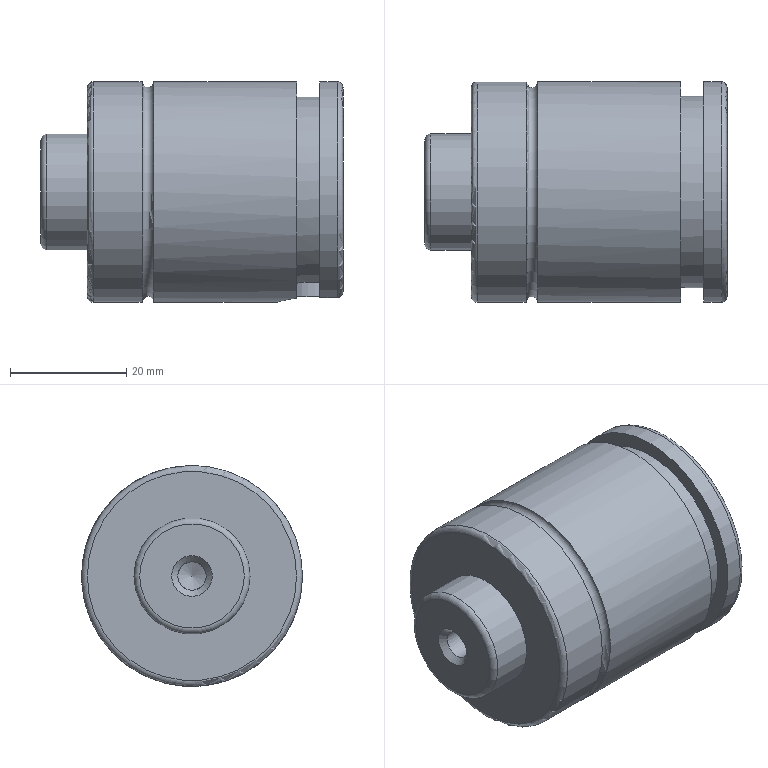Part | NX | features 1 2 | 1 solid | 34 faces | box 52 x 38 x 38 mm | volume 50464 mm3 | plane 16 | cylinder 10 | torus 4 | cone 4 | commonest cylinder face diameters 4.9 x3 38 x3 9.5 x1 11 x1 20 x1 33 x1
STEP:
#1=CARTESIAN_POINT('',(-1488.5,-459.,-300.));
#2=VERTEX_POINT('',#1);
#3=CARTESIAN_POINT('',(-1488.5,-440.,-300.));
#4=DIRECTION('',(1.,0.,0.));
#5=DIRECTION('',(0.,-1.,0.));
#6=AXIS2_PLACEMENT_3D('',#3,#4,#5);
#7=CIRCLE('',#6,19.);
#8=EDGE_CURVE('',#2,#2,#7,.T.);
#9=ORIENTED_EDGE('',*,*,#8,.F.);
#10=EDGE_LOOP('',(#9));
#11=FACE_BOUND('',#10,.T.);
#12=CARTESIAN_POINT('',(-1490.5,-459.,-300.));
#13=VERTEX_POINT('',#12);
#14=CARTESIAN_POINT('',(-1490.5,-440.,-300.));
#15=DIRECTION('',(1.,0.,0.));
#16=DIRECTION('',(0.,-1.,0.));
#17=AXIS2_PLACEMENT_3D('',#14,#15,#16);
#18=CIRCLE('',#17,19.);
#19=EDGE_CURVE('',#13,#13,#18,.T.);
#20=ORIENTED_EDGE('',*,*,#19,.T.);
#21=EDGE_LOOP('',(#20));
#22=FACE_BOUND('',#21,.T.);
#23=CARTESIAN_POINT('',(-1489.5,-440.,-300.));
#24=DIRECTION('',(-1.,0.,0.));
#25=DIRECTION('',(0.,0.,1.));
#26=AXIS2_PLACEMENT_3D('',#23,#24,#25);
#27=TOROIDAL_SURFACE('',#26,19.,1.);
#28=ADVANCED_FACE('',(#11,#22),#27,.F.);
#29=CARTESIAN_POINT('',(-1498.9,-459.,-300.));
#30=VERTEX_POINT('',#29);
#31=CARTESIAN_POINT('',(-1498.9,-440.,-300.));
#32=DIRECTION('',(1.,0.,0.));
#33=DIRECTION('',(0.,-1.,0.));
#34=AXIS2_PLACEMENT_3D('',#31,#32,#33);
#35=CIRCLE('',#34,19.);
#36=EDGE_CURVE('',#30,#30,#35,.T.);
#37=ORIENTED_EDGE('',*,*,#36,.F.);
#38=EDGE_LOOP('',(#37));
#39=FACE_BOUND('',#38,.T.);
#40=CARTESIAN_POINT('',(-1499.9,-458.,-300.));
#41=VERTEX_POINT('',#40);
#42=CARTESIAN_POINT('',(-1499.9,-440.,-300.));
#43=DIRECTION('',(1.,0.,0.));
#44=DIRECTION('',(0.,-1.,0.));
#45=AXIS2_PLACEMENT_3D('',#42,#43,#44);
#46=CIRCLE('',#45,18.);
#47=EDGE_CURVE('',#41,#41,#46,.T.);
#48=ORIENTED_EDGE('',*,*,#47,.T.);
#49=EDGE_LOOP('',(#48));
#50=FACE_BOUND('',#49,.T.);
#51=CARTESIAN_POINT('',(-1498.9,-440.,-300.));
#52=DIRECTION('',(-1.,0.,0.));
#53=DIRECTION('',(0.,0.,1.));
#54=AXIS2_PLACEMENT_3D('',#51,#52,#53);
#55=TOROIDAL_SURFACE('',#54,18.,1.);
#56=ADVANCED_FACE('',(#39,#50),#55,.T.);
#57=ORIENTED_EDGE('',*,*,#19,.F.);
#58=EDGE_LOOP('',(#57));
#59=FACE_BOUND('',#58,.T.);
#60=ORIENTED_EDGE('',*,*,#36,.T.);
#61=EDGE_LOOP('',(#60));
#62=FACE_BOUND('',#61,.T.);
#63=CARTESIAN_POINT('',(-1494.7,-440.,-300.));
#64=DIRECTION('',(1.,0.,0.));
#65=DIRECTION('',(0.,0.,-1.));
#66=AXIS2_PLACEMENT_3D('',#63,#64,#65);
#67=CYLINDRICAL_SURFACE('',#66,19.);
#68=ADVANCED_FACE('',(#59,#62),#67,.T.);
#69=CARTESIAN_POINT('',(-1506.9,-450.,-300.));
#70=VERTEX_POINT('',#69);
#71=CARTESIAN_POINT('',(-1506.9,-440.,-300.));
#72=DIRECTION('',(1.,0.,0.));
#73=DIRECTION('',(0.,-1.,0.));
#74=AXIS2_PLACEMENT_3D('',#71,#72,#73);
#75=CIRCLE('',#74,10.);
#76=EDGE_CURVE('',#70,#70,#75,.T.);
#77=ORIENTED_EDGE('',*,*,#76,.F.);
#78=EDGE_LOOP('',(#77));
#79=FACE_BOUND('',#78,.T.);
#80=CARTESIAN_POINT('',(-1507.9,-449.,-300.));
#81=VERTEX_POINT('',#80);
#82=CARTESIAN_POINT('',(-1507.9,-440.,-300.));
#83=DIRECTION('',(1.,0.,0.));
#84=DIRECTION('',(0.,-1.,0.));
#85=AXIS2_PLACEMENT_3D('',#82,#83,#84);
#86=CIRCLE('',#85,9.);
#87=EDGE_CURVE('',#81,#81,#86,.T.);
#88=ORIENTED_EDGE('',*,*,#87,.T.);
#89=EDGE_LOOP('',(#88));
#90=FACE_BOUND('',#89,.T.);
#91=CARTESIAN_POINT('',(-1506.9,-440.,-300.));
#92=DIRECTION('',(-1.,0.,0.));
#93=DIRECTION('',(0.,0.,1.));
#94=AXIS2_PLACEMENT_3D('',#91,#92,#93);
#95=TOROIDAL_SURFACE('',#94,9.,1.);
#96=ADVANCED_FACE('',(#79,#90),#95,.T.);
#97=CARTESIAN_POINT('',(-1499.9,-450.,-300.));
#98=VERTEX_POINT('',#97);
#99=CARTESIAN_POINT('',(-1499.9,-440.,-300.));
#100=DIRECTION('',(-1.,0.,0.));
#101=DIRECTION('',(0.,-1.,0.));
#102=AXIS2_PLACEMENT_3D('',#99,#100,#101);
#103=CIRCLE('',#102,10.);
#104=EDGE_CURVE('',#98,#98,#103,.T.);
#105=ORIENTED_EDGE('',*,*,#104,.T.);
#106=EDGE_LOOP('',(#105));
#107=FACE_BOUND('',#106,.T.);
#108=ORIENTED_EDGE('',*,*,#76,.T.);
#109=EDGE_LOOP('',(#108));
#110=FACE_BOUND('',#109,.T.);
#111=CARTESIAN_POINT('',(-1503.4,-440.,-300.));
#112=DIRECTION('',(1.,0.,0.));
#113=DIRECTION('',(0.,0.,-1.));
#114=AXIS2_PLACEMENT_3D('',#111,#112,#113);
#115=CYLINDRICAL_SURFACE('',#114,10.);
#116=ADVANCED_FACE('',(#107,#110),#115,.T.);
#117=CARTESIAN_POINT('',(-1455.9,-450.05,-300.));
#118=VERTEX_POINT('',#117);
#119=CARTESIAN_POINT('',(-1455.9,-452.5,-300.));
#120=DIRECTION('',(1.,0.,0.));
#121=DIRECTION('',(0.,1.,0.));
#122=AXIS2_PLACEMENT_3D('',#119,#120,#121);
#123=CIRCLE('',#122,2.45);
#124=EDGE_CURVE('',#118,#118,#123,.T.);
#125=ORIENTED_EDGE('',*,*,#124,.T.);
#126=EDGE_LOOP('',(#125));
#127=FACE_BOUND('',#126,.T.);
#128=CARTESIAN_POINT('',(-1463.1,-450.05,-300.));
#129=VERTEX_POINT('',#128);
#130=CARTESIAN_POINT('',(-1463.1,-452.5,-300.));
#131=DIRECTION('',(-1.,0.,0.));
#132=DIRECTION('',(0.,1.,0.));
#133=AXIS2_PLACEMENT_3D('',#130,#131,#132);
#134=CIRCLE('',#133,2.45);
#135=EDGE_CURVE('',#129,#129,#134,.T.);
#136=ORIENTED_EDGE('',*,*,#135,.T.);
#137=EDGE_LOOP('',(#136));
#138=FACE_BOUND('',#137,.T.);
#139=CARTESIAN_POINT('',(-1459.5,-452.5,-300.));
#140=DIRECTION('',(-1.,0.,0.));
#141=DIRECTION('',(0.,0.,1.));
#142=AXIS2_PLACEMENT_3D('',#139,#140,#141);
#143=CYLINDRICAL_SURFACE('',#142,2.45);
#144=ADVANCED_FACE('',(#127,#138),#143,.F.);
#145=CARTESIAN_POINT('',(-1464.4,-452.5,-300.));
#146=VERTEX_POINT('',#145);
#147=VERTEX_LOOP('',#146);
#148=FACE_BOUND('',#147,.T.);
#149=ORIENTED_EDGE('',*,*,#135,.F.);
#150=EDGE_LOOP('',(#149));
#151=FACE_BOUND('',#150,.T.);
#152=CARTESIAN_POINT('',(-1463.75,-452.5,-300.));
#153=DIRECTION('',(1.,0.,0.));
#154=DIRECTION('',(0.,0.,-1.));
#155=AXIS2_PLACEMENT_3D('',#152,#153,#154);
#156=CONICAL_SURFACE('',#155,1.225,1.083);
#157=ADVANCED_FACE('',(#148,#151),#156,.F.);
#158=CARTESIAN_POINT('',(-1507.9,-443.5,-300.));
#159=VERTEX_POINT('',#158);
#160=CARTESIAN_POINT('',(-1507.9,-440.,-300.));
#161=DIRECTION('',(-1.,0.,0.));
#162=DIRECTION('',(0.,-1.,0.));
#163=AXIS2_PLACEMENT_3D('',#160,#161,#162);
#164=CIRCLE('',#163,3.5);
#165=EDGE_CURVE('',#159,#159,#164,.T.);
#166=ORIENTED_EDGE('',*,*,#165,.T.);
#167=EDGE_LOOP('',(#166));
#168=FACE_BOUND('',#167,.T.);
#169=CARTESIAN_POINT('',(-1506.85,-442.45,-300.));
#170=VERTEX_POINT('',#169);
#171=CARTESIAN_POINT('',(-1506.85,-440.,-300.));
#172=DIRECTION('',(1.,0.,0.));
#173=DIRECTION('',(0.,-1.,0.));
#174=AXIS2_PLACEMENT_3D('',#171,#172,#173);
#175=CIRCLE('',#174,2.45);
#176=EDGE_CURVE('',#170,#170,#175,.T.);
#177=ORIENTED_EDGE('',*,*,#176,.T.);
#178=EDGE_LOOP('',(#177));
#179=FACE_BOUND('',#178,.T.);
#180=CARTESIAN_POINT('',(-1507.375,-440.,-300.));
#181=DIRECTION('',(-1.,0.,0.));
#182=DIRECTION('',(0.,0.,1.));
#183=AXIS2_PLACEMENT_3D('',#180,#181,#182);
#184=CONICAL_SURFACE('',#183,2.975,0.7854);
#185=ADVANCED_FACE('',(#168,#179),#184,.F.);
#186=ORIENTED_EDGE('',*,*,#176,.F.);
#187=EDGE_LOOP('',(#186));
#188=FACE_BOUND('',#187,.T.);
#189=CARTESIAN_POINT('',(-1501.4,-442.45,-300.));
#190=VERTEX_POINT('',#189);
#191=CARTESIAN_POINT('',(-1501.4,-440.,-300.));
#192=DIRECTION('',(1.,0.,0.));
#193=DIRECTION('',(0.,-1.,0.));
#194=AXIS2_PLACEMENT_3D('',#191,#192,#193);
#195=CIRCLE('',#194,2.45);
#196=EDGE_CURVE('',#190,#190,#195,.T.);
#197=ORIENTED_EDGE('',*,*,#196,.T.);
#198=EDGE_LOOP('',(#197));
#199=FACE_BOUND('',#198,.T.);
#200=CARTESIAN_POINT('',(-1504.125,-440.,-300.));
#201=DIRECTION('',(1.,0.,0.));
#202=DIRECTION('',(0.,0.,-1.));
#203=AXIS2_PLACEMENT_3D('',#200,#201,#202);
#204=CYLINDRICAL_SURFACE('',#203,2.45);
#205=ADVANCED_FACE('',(#188,#199),#204,.F.);
#206=CARTESIAN_POINT('',(-1500.4,-440.,-300.));
#207=VERTEX_POINT('',#206);
#208=VERTEX_LOOP('',#207);
#209=FACE_BOUND('',#208,.T.);
#210=ORIENTED_EDGE('',*,*,#196,.F.);
#211=EDGE_LOOP('',(#210));
#212=FACE_BOUND('',#211,.T.);
#213=CARTESIAN_POINT('',(-1500.9,-440.,-300.));
#214=DIRECTION('',(-1.,0.,0.));
#215=DIRECTION('',(0.,0.,1.));
#216=AXIS2_PLACEMENT_3D('',#213,#214,#215);
#217=CONICAL_SURFACE('',#216,1.225,1.183);
#218=ADVANCED_FACE('',(#209,#212),#217,.F.);
#219=CARTESIAN_POINT('',(-1463.1,-429.95,-300.));
#220=VERTEX_POINT('',#219);
#221=CARTESIAN_POINT('',(-1463.1,-427.5,-300.));
#222=DIRECTION('',(1.,0.,0.));
#223=DIRECTION('',(0.,-1.,0.));
#224=AXIS2_PLACEMENT_3D('',#221,#222,#223);
#225=CIRCLE('',#224,2.45);
#226=EDGE_CURVE('',#220,#220,#225,.T.);
#227=ORIENTED_EDGE('',*,*,#226,.T.);
#228=EDGE_LOOP('',(#227));
#229=FACE_BOUND('',#228,.T.);
#230=CARTESIAN_POINT('',(-1464.4,-427.5,-300.));
#231=VERTEX_POINT('',#230);
#232=VERTEX_LOOP('',#231);
#233=FACE_BOUND('',#232,.T.);
#234=CARTESIAN_POINT('',(-1463.75,-427.5,-300.));
#235=DIRECTION('',(1.,0.,0.));
#236=DIRECTION('',(0.,0.,-1.));
#237=AXIS2_PLACEMENT_3D('',#234,#235,#236);
#238=CONICAL_SURFACE('',#237,1.225,1.083);
#239=ADVANCED_FACE('',(#229,#233),#238,.F.);
#240=ORIENTED_EDGE('',*,*,#226,.F.);
#241=EDGE_LOOP('',(#240));
#242=FACE_BOUND('',#241,.T.);
#243=CARTESIAN_POINT('',(-1455.9,-429.95,-300.));
#244=VERTEX_POINT('',#243);
#245=CARTESIAN_POINT('',(-1455.9,-427.5,-300.));
#246=DIRECTION('',(1.,0.,0.));
#247=DIRECTION('',(0.,-1.,0.));
#248=AXIS2_PLACEMENT_3D('',#245,#246,#247);
#249=CIRCLE('',#248,2.45);
#250=EDGE_CURVE('',#244,#244,#249,.T.);
#251=ORIENTED_EDGE('',*,*,#250,.T.);
#252=EDGE_LOOP('',(#251));
#253=FACE_BOUND('',#252,.T.);
#254=CARTESIAN_POINT('',(-1459.5,-427.5,-300.));
#255=DIRECTION('',(1.,0.,0.));
#256=DIRECTION('',(0.,0.,-1.));
#257=AXIS2_PLACEMENT_3D('',#254,#255,#256);
#258=CYLINDRICAL_SURFACE('',#257,2.45);
#259=ADVANCED_FACE('',(#242,#253),#258,.F.);
#260=CARTESIAN_POINT('',(-1456.9,-434.5,-318.187));
#261=VERTEX_POINT('',#260);
#262=CARTESIAN_POINT('',(-1456.9,-445.5,-318.187));
#263=VERTEX_POINT('',#262);
#264=CARTESIAN_POINT('',(-1456.9,-440.,-300.));
#265=DIRECTION('',(1.,0.,0.));
#266=DIRECTION('',(0.,-1.,0.));
#267=AXIS2_PLACEMENT_3D('',#264,#265,#266);
#268=CIRCLE('',#267,19.);
#269=EDGE_CURVE('',#261,#263,#268,.T.);
#270=ORIENTED_EDGE('',*,*,#269,.F.);
#271=CARTESIAN_POINT('',(-1459.9,-434.5,-318.187));
#272=VERTEX_POINT('',#271);
#273=CARTESIAN_POINT('',(-1458.4,-434.5,-318.187));
#274=DIRECTION('',(1.,0.,0.));
#275=VECTOR('',#274,1000.);
#276=LINE('',#273,#275);
#277=EDGE_CURVE('',#272,#261,#276,.T.);
#278=ORIENTED_EDGE('',*,*,#277,.F.);
#279=CARTESIAN_POINT('',(-1459.9,-445.5,-318.187));
#280=VERTEX_POINT('',#279);
#281=CARTESIAN_POINT('',(-1459.9,-440.,-300.));
#282=DIRECTION('',(-1.,0.,0.));
#283=DIRECTION('',(0.,-1.,0.));
#284=AXIS2_PLACEMENT_3D('',#281,#282,#283);
#285=CIRCLE('',#284,19.);
#286=EDGE_CURVE('',#280,#272,#285,.T.);
#287=ORIENTED_EDGE('',*,*,#286,.F.);
#288=CARTESIAN_POINT('',(-1458.4,-445.5,-318.187));
#289=DIRECTION('',(-1.,0.,0.));
#290=VECTOR('',#289,1000.);
#291=LINE('',#288,#290);
#292=EDGE_CURVE('',#263,#280,#291,.T.);
#293=ORIENTED_EDGE('',*,*,#292,.F.);
#294=EDGE_LOOP('',(#270,#278,#287,#293));
#295=FACE_BOUND('',#294,.T.);
#296=CARTESIAN_POINT('',(-1472.7,-440.,-300.));
#297=DIRECTION('',(1.,0.,0.));
#298=DIRECTION('',(0.,0.,-1.));
#299=AXIS2_PLACEMENT_3D('',#296,#297,#298);
#300=CYLINDRICAL_SURFACE('',#299,19.);
#301=ADVANCED_FACE('',(#295),#300,.T.);
#302=CARTESIAN_POINT('',(-1455.9,-445.5,-317.139));
#303=VERTEX_POINT('',#302);
#304=CARTESIAN_POINT('',(-1455.9,-445.5,-317.139));
#305=CARTESIAN_POINT('',(-1455.9,-445.5,-317.68));
#306=CARTESIAN_POINT('',(-1456.358,-445.5,-318.187));
#307=CARTESIAN_POINT('',(-1456.9,-445.5,-318.187));
#308=B_SPLINE_CURVE_WITH_KNOTS('',3,(#304,#305,#306,#307),.UNSPECIFIED.,.F.,.F.,(4,4),(0.,0.0016),.UNSPECIFIED.);
#309=EDGE_CURVE('',#303,#263,#308,.T.);
#310=ORIENTED_EDGE('',*,*,#309,.F.);
#311=CARTESIAN_POINT('',(-1455.9,-434.5,-317.139));
#312=VERTEX_POINT('',#311);
#313=CARTESIAN_POINT('',(-1455.9,-440.,-300.));
#314=DIRECTION('',(1.,0.,0.));
#315=DIRECTION('',(0.,-1.,0.));
#316=AXIS2_PLACEMENT_3D('',#313,#314,#315);
#317=CIRCLE('',#316,18.);
#318=EDGE_CURVE('',#312,#303,#317,.T.);
#319=ORIENTED_EDGE('',*,*,#318,.F.);
#320=CARTESIAN_POINT('',(-1456.9,-434.5,-318.187));
#321=CARTESIAN_POINT('',(-1456.359,-434.5,-318.187));
#322=CARTESIAN_POINT('',(-1455.9,-434.5,-317.68));
#323=CARTESIAN_POINT('',(-1455.9,-434.5,-317.139));
#324=B_SPLINE_CURVE_WITH_KNOTS('',3,(#320,#321,#322,#323),.UNSPECIFIED.,.F.,.F.,(4,4),(0.,0.0016),.UNSPECIFIED.);
#325=EDGE_CURVE('',#261,#312,#324,.T.);
#326=ORIENTED_EDGE('',*,*,#325,.F.);
#327=ORIENTED_EDGE('',*,*,#269,.T.);
#328=EDGE_LOOP('',(#310,#319,#326,#327));
#329=FACE_BOUND('',#328,.T.);
#330=CARTESIAN_POINT('',(-1456.9,-440.,-300.));
#331=DIRECTION('',(-1.,0.,0.));
#332=DIRECTION('',(0.,0.,1.));
#333=AXIS2_PLACEMENT_3D('',#330,#331,#332);
#334=TOROIDAL_SURFACE('',#333,18.,1.);
#335=ADVANCED_FACE('',(#329),#334,.T.);
#336=CARTESIAN_POINT('',(-1459.9,-434.5,-315.556));
#337=VERTEX_POINT('',#336);
#338=CARTESIAN_POINT('',(-1459.9,-445.5,-315.556));
#339=VERTEX_POINT('',#338);
#340=CARTESIAN_POINT('',(-1459.9,-440.,-300.));
#341=DIRECTION('',(1.,0.,0.));
#342=DIRECTION('',(0.,-1.,0.));
#343=AXIS2_PLACEMENT_3D('',#340,#341,#342);
#344=CIRCLE('',#343,16.5);
#345=EDGE_CURVE('',#337,#339,#344,.T.);
#346=ORIENTED_EDGE('',*,*,#345,.F.);
#347=CARTESIAN_POINT('',(-1461.9,-434.5,-315.556));
#348=VERTEX_POINT('',#347);
#349=CARTESIAN_POINT('',(-1460.9,-434.5,-315.556));
#350=DIRECTION('',(1.,0.,0.));
#351=VECTOR('',#350,1000.);
#352=LINE('',#349,#351);
#353=EDGE_CURVE('',#348,#337,#352,.T.);
#354=ORIENTED_EDGE('',*,*,#353,.F.);
#355=CARTESIAN_POINT('',(-1463.9,-434.877,-315.684));
#356=VERTEX_POINT('',#355);
#357=CARTESIAN_POINT('',(-1463.9,-434.877,-315.684));
#358=CARTESIAN_POINT('',(-1463.259,-434.626,-315.603));
#359=CARTESIAN_POINT('',(-1462.593,-434.5,-315.556));
#360=CARTESIAN_POINT('',(-1461.9,-434.5,-315.556));
#361=B_SPLINE_CURVE_WITH_KNOTS('',3,(#357,#358,#359,#360),.UNSPECIFIED.,.F.,.F.,(4,4),(0.,0.002039),.UNSPECIFIED.);
#362=EDGE_CURVE('',#356,#348,#361,.T.);
#363=ORIENTED_EDGE('',*,*,#362,.F.);
#364=CARTESIAN_POINT('',(-1463.9,-445.123,-315.684));
#365=VERTEX_POINT('',#364);
#366=CARTESIAN_POINT('',(-1463.9,-440.,-300.));
#367=DIRECTION('',(1.,0.,0.));
#368=DIRECTION('',(0.,-1.,0.));
#369=AXIS2_PLACEMENT_3D('',#366,#367,#368);
#370=CIRCLE('',#369,16.5);
#371=EDGE_CURVE('',#356,#365,#370,.T.);
#372=ORIENTED_EDGE('',*,*,#371,.T.);
#373=CARTESIAN_POINT('',(-1461.9,-445.5,-315.556));
#374=VERTEX_POINT('',#373);
#375=CARTESIAN_POINT('',(-1461.9,-445.5,-315.556));
#376=CARTESIAN_POINT('',(-1462.593,-445.5,-315.556));
#377=CARTESIAN_POINT('',(-1463.259,-445.374,-315.603));
#378=CARTESIAN_POINT('',(-1463.9,-445.123,-315.684));
#379=B_SPLINE_CURVE_WITH_KNOTS('',3,(#375,#376,#377,#378),.UNSPECIFIED.,.F.,.F.,(4,4),(0.,0.002039),.UNSPECIFIED.);
#380=EDGE_CURVE('',#374,#365,#379,.T.);
#381=ORIENTED_EDGE('',*,*,#380,.F.);
#382=CARTESIAN_POINT('',(-1460.9,-445.5,-315.556));
#383=DIRECTION('',(-1.,0.,0.));
#384=VECTOR('',#383,1000.);
#385=LINE('',#382,#384);
#386=EDGE_CURVE('',#339,#374,#385,.T.);
#387=ORIENTED_EDGE('',*,*,#386,.F.);
#388=EDGE_LOOP('',(#346,#354,#363,#372,#381,#387));
#389=FACE_BOUND('',#388,.T.);
#390=CARTESIAN_POINT('',(-1461.9,-440.,-300.));
#391=DIRECTION('',(1.,0.,0.));
#392=DIRECTION('',(0.,0.,-1.));
#393=AXIS2_PLACEMENT_3D('',#390,#391,#392);
#394=CYLINDRICAL_SURFACE('',#393,16.5);
#395=ADVANCED_FACE('',(#389),#394,.T.);
#396=CARTESIAN_POINT('',(-1463.9,-445.123,-318.296));
#397=VERTEX_POINT('',#396);
#398=CARTESIAN_POINT('',(-1463.9,-434.877,-318.296));
#399=VERTEX_POINT('',#398);
#400=CARTESIAN_POINT('',(-1463.9,-445.123,-318.296));
#401=CARTESIAN_POINT('',(-1464.934,-444.72,-318.409));
#402=CARTESIAN_POINT('',(-1466.701,-443.317,-318.782));
#403=CARTESIAN_POINT('',(-1467.747,-439.998,-319.109));
#404=CARTESIAN_POINT('',(-1466.711,-436.7,-318.784));
#405=CARTESIAN_POINT('',(-1464.934,-435.28,-318.409));
#406=CARTESIAN_POINT('',(-1463.9,-434.877,-318.296));
#407=B_SPLINE_CURVE_WITH_KNOTS('',3,(#400,#401,#402,#403,#404,#405,#406),.UNSPECIFIED.,.F.,.F.,(4,1,1,1,4),(0.,0.003298,0.006596,0.009894,0.01319),.UNSPECIFIED.);
#408=EDGE_CURVE('',#397,#399,#407,.T.);
#409=ORIENTED_EDGE('',*,*,#408,.F.);
#410=CARTESIAN_POINT('',(-1463.9,-440.,-300.));
#411=DIRECTION('',(1.,0.,0.));
#412=DIRECTION('',(0.,-1.,0.));
#413=AXIS2_PLACEMENT_3D('',#410,#411,#412);
#414=CIRCLE('',#413,19.);
#415=EDGE_CURVE('',#399,#397,#414,.T.);
#416=ORIENTED_EDGE('',*,*,#415,.F.);
#417=EDGE_LOOP('',(#409,#416));
#418=FACE_BOUND('',#417,.T.);
#419=ORIENTED_EDGE('',*,*,#8,.T.);
#420=EDGE_LOOP('',(#419));
#421=FACE_BOUND('',#420,.T.);
#422=CARTESIAN_POINT('',(-1472.7,-440.,-300.));
#423=DIRECTION('',(1.,0.,0.));
#424=DIRECTION('',(0.,0.,-1.));
#425=AXIS2_PLACEMENT_3D('',#422,#423,#424);
#426=CYLINDRICAL_SURFACE('',#425,19.);
#427=ADVANCED_FACE('',(#418,#421),#426,.T.);
#428=CARTESIAN_POINT('',(-1461.9,-444.75,-314.5));
#429=VERTEX_POINT('',#428);
#430=CARTESIAN_POINT('',(-1461.9,-440.,-314.5));
#431=DIRECTION('',(0.,0.,-1.));
#432=DIRECTION('',(0.,-1.,0.));
#433=AXIS2_PLACEMENT_3D('',#430,#431,#432);
#434=CIRCLE('',#433,4.75);
#435=EDGE_CURVE('',#429,#429,#434,.T.);
#436=ORIENTED_EDGE('',*,*,#435,.T.);
#437=EDGE_LOOP('',(#436));
#438=FACE_BOUND('',#437,.T.);
#439=CARTESIAN_POINT('',(-1461.9,-444.75,-318.));
#440=VERTEX_POINT('',#439);
#441=CARTESIAN_POINT('',(-1461.9,-440.,-318.));
#442=DIRECTION('',(0.,0.,-1.));
#443=DIRECTION('',(0.,-1.,0.));
#444=AXIS2_PLACEMENT_3D('',#441,#442,#443);
#445=CIRCLE('',#444,4.75);
#446=EDGE_CURVE('',#440,#440,#445,.T.);
#447=ORIENTED_EDGE('',*,*,#446,.F.);
#448=EDGE_LOOP('',(#447));
#449=FACE_BOUND('',#448,.T.);
#450=CARTESIAN_POINT('',(-1461.9,-440.,-300.));
#451=DIRECTION('',(0.,0.,1.));
#452=DIRECTION('',(0.,-1.,0.));
#453=AXIS2_PLACEMENT_3D('',#450,#451,#452);
#454=CYLINDRICAL_SURFACE('',#453,4.75);
#455=ADVANCED_FACE('',(#438,#449),#454,.T.);
#456=CARTESIAN_POINT('',(-1461.034,-441.5,-313.));
#457=VERTEX_POINT('',#456);
#458=CARTESIAN_POINT('',(-1460.168,-440.,-313.));
#459=VERTEX_POINT('',#458);
#460=CARTESIAN_POINT('',(-1461.034,-441.5,-313.));
#461=DIRECTION('',(0.5,0.866,0.));
#462=VECTOR('',#461,1000.);
#463=LINE('',#460,#462);
#464=EDGE_CURVE('',#457,#459,#463,.T.);
#465=ORIENTED_EDGE('',*,*,#464,.T.);
#466=CARTESIAN_POINT('',(-1460.168,-440.,-318.));
#467=VERTEX_POINT('',#466);
#468=CARTESIAN_POINT('',(-1460.168,-440.,-318.));
#469=DIRECTION('',(0.,0.,1.));
#470=VECTOR('',#469,1000.);
#471=LINE('',#468,#470);
#472=EDGE_CURVE('',#467,#459,#471,.T.);
#473=ORIENTED_EDGE('',*,*,#472,.F.);
#474=CARTESIAN_POINT('',(-1461.034,-441.5,-318.));
#475=VERTEX_POINT('',#474);
#476=CARTESIAN_POINT('',(-1460.067,-439.826,-318.));
#477=DIRECTION('',(-0.5,-0.866,0.));
#478=VECTOR('',#477,1000.);
#479=LINE('',#476,#478);
#480=EDGE_CURVE('',#467,#475,#479,.T.);
#481=ORIENTED_EDGE('',*,*,#480,.T.);
#482=CARTESIAN_POINT('',(-1461.034,-441.5,-318.));
#483=DIRECTION('',(0.,0.,1.));
#484=VECTOR('',#483,1000.);
#485=LINE('',#482,#484);
#486=EDGE_CURVE('',#475,#457,#485,.T.);
#487=ORIENTED_EDGE('',*,*,#486,.T.);
#488=EDGE_LOOP('',(#465,#473,#481,#487));
#489=FACE_BOUND('',#488,.T.);
#490=CARTESIAN_POINT('',(-1461.034,-441.5,-318.));
#491=DIRECTION('',(0.866,-0.5,0.));
#492=DIRECTION('',(-0.5,-0.866,0.));
#493=AXIS2_PLACEMENT_3D('',#490,#491,#492);
#494=PLANE('',#493);
#495=ADVANCED_FACE('',(#489),#494,.F.);
#496=CARTESIAN_POINT('',(-1461.034,-438.5,-313.));
#497=VERTEX_POINT('',#496);
#498=CARTESIAN_POINT('',(-1460.168,-440.,-313.));
#499=DIRECTION('',(-0.5,0.866,0.));
#500=VECTOR('',#499,1000.);
#501=LINE('',#498,#500);
#502=EDGE_CURVE('',#459,#497,#501,.T.);
#503=ORIENTED_EDGE('',*,*,#502,.T.);
#504=CARTESIAN_POINT('',(-1461.034,-438.5,-318.));
#505=VERTEX_POINT('',#504);
#506=CARTESIAN_POINT('',(-1461.034,-438.5,-318.));
#507=DIRECTION('',(0.,0.,1.));
#508=VECTOR('',#507,1000.);
#509=LINE('',#506,#508);
#510=EDGE_CURVE('',#505,#497,#509,.T.);
#511=ORIENTED_EDGE('',*,*,#510,.F.);
#512=CARTESIAN_POINT('',(-1459.634,-440.924,-318.));
#513=DIRECTION('',(0.5,-0.866,0.));
#514=VECTOR('',#513,1000.);
#515=LINE('',#512,#514);
#516=EDGE_CURVE('',#505,#467,#515,.T.);
#517=ORIENTED_EDGE('',*,*,#516,.T.);
#518=ORIENTED_EDGE('',*,*,#472,.T.);
#519=EDGE_LOOP('',(#503,#511,#517,#518));
#520=FACE_BOUND('',#519,.T.);
#521=CARTESIAN_POINT('',(-1460.168,-440.,-318.));
#522=DIRECTION('',(0.866,0.5,0.));
#523=DIRECTION('',(0.5,-0.866,0.));
#524=AXIS2_PLACEMENT_3D('',#521,#522,#523);
#525=PLANE('',#524);
#526=ADVANCED_FACE('',(#520),#525,.F.);
#527=CARTESIAN_POINT('',(-1462.766,-438.5,-313.));
#528=VERTEX_POINT('',#527);
#529=CARTESIAN_POINT('',(-1461.034,-438.5,-313.));
#530=DIRECTION('',(-1.,0.,0.));
#531=VECTOR('',#530,1000.);
#532=LINE('',#529,#531);
#533=EDGE_CURVE('',#497,#528,#532,.T.);
#534=ORIENTED_EDGE('',*,*,#533,.T.);
#535=CARTESIAN_POINT('',(-1462.766,-438.5,-318.));
#536=VERTEX_POINT('',#535);
#537=CARTESIAN_POINT('',(-1462.766,-438.5,-318.));
#538=DIRECTION('',(0.,0.,1.));
#539=VECTOR('',#538,1000.);
#540=LINE('',#537,#539);
#541=EDGE_CURVE('',#536,#528,#540,.T.);
#542=ORIENTED_EDGE('',*,*,#541,.F.);
#543=CARTESIAN_POINT('',(-1458.467,-438.5,-318.));
#544=DIRECTION('',(1.,0.,0.));
#545=VECTOR('',#544,1000.);
#546=LINE('',#543,#545);
#547=EDGE_CURVE('',#536,#505,#546,.T.);
#548=ORIENTED_EDGE('',*,*,#547,.T.);
#549=ORIENTED_EDGE('',*,*,#510,.T.);
#550=EDGE_LOOP('',(#534,#542,#548,#549));
#551=FACE_BOUND('',#550,.T.);
#552=CARTESIAN_POINT('',(-1461.034,-438.5,-318.));
#553=DIRECTION('',(0.,1.,0.));
#554=DIRECTION('',(0.,0.,1.));
#555=AXIS2_PLACEMENT_3D('',#552,#553,#554);
#556=PLANE('',#555);
#557=ADVANCED_FACE('',(#551),#556,.F.);
#558=CARTESIAN_POINT('',(-1463.632,-440.,-313.));
#559=VERTEX_POINT('',#558);
#560=CARTESIAN_POINT('',(-1462.766,-438.5,-313.));
#561=DIRECTION('',(-0.5,-0.866,0.));
#562=VECTOR('',#561,1000.);
#563=LINE('',#560,#562);
#564=EDGE_CURVE('',#528,#559,#563,.T.);
#565=ORIENTED_EDGE('',*,*,#564,.T.);
#566=CARTESIAN_POINT('',(-1463.632,-440.,-318.));
#567=VERTEX_POINT('',#566);
#568=CARTESIAN_POINT('',(-1463.632,-440.,-318.));
#569=DIRECTION('',(0.,0.,1.));
#570=VECTOR('',#569,1000.);
#571=LINE('',#568,#570);
#572=EDGE_CURVE('',#567,#559,#571,.T.);
#573=ORIENTED_EDGE('',*,*,#572,.F.);
#574=CARTESIAN_POINT('',(-1462.233,-437.576,-318.));
#575=DIRECTION('',(0.5,0.866,0.));
#576=VECTOR('',#575,1000.);
#577=LINE('',#574,#576);
#578=EDGE_CURVE('',#567,#536,#577,.T.);
#579=ORIENTED_EDGE('',*,*,#578,.T.);
#580=ORIENTED_EDGE('',*,*,#541,.T.);
#581=EDGE_LOOP('',(#565,#573,#579,#580));
#582=FACE_BOUND('',#581,.T.);
#583=CARTESIAN_POINT('',(-1462.766,-438.5,-318.));
#584=DIRECTION('',(-0.866,0.5,0.));
#585=DIRECTION('',(0.5,0.866,0.));
#586=AXIS2_PLACEMENT_3D('',#583,#584,#585);
#587=PLANE('',#586);
#588=ADVANCED_FACE('',(#582),#587,.F.);
#589=CARTESIAN_POINT('',(-1462.766,-441.5,-313.));
#590=VERTEX_POINT('',#589);
#591=CARTESIAN_POINT('',(-1463.632,-440.,-313.));
#592=DIRECTION('',(0.5,-0.866,0.));
#593=VECTOR('',#592,1000.);
#594=LINE('',#591,#593);
#595=EDGE_CURVE('',#559,#590,#594,.T.);
#596=ORIENTED_EDGE('',*,*,#595,.T.);
#597=CARTESIAN_POINT('',(-1462.766,-441.5,-318.));
#598=VERTEX_POINT('',#597);
#599=CARTESIAN_POINT('',(-1462.766,-441.5,-318.));
#600=DIRECTION('',(0.,0.,1.));
#601=VECTOR('',#600,1000.);
#602=LINE('',#599,#601);
#603=EDGE_CURVE('',#598,#590,#602,.T.);
#604=ORIENTED_EDGE('',*,*,#603,.F.);
#605=CARTESIAN_POINT('',(-1462.666,-441.674,-318.));
#606=DIRECTION('',(-0.5,0.866,0.));
#607=VECTOR('',#606,1000.);
#608=LINE('',#605,#607);
#609=EDGE_CURVE('',#598,#567,#608,.T.);
#610=ORIENTED_EDGE('',*,*,#609,.T.);
#611=ORIENTED_EDGE('',*,*,#572,.T.);
#612=EDGE_LOOP('',(#596,#604,#610,#611));
#613=FACE_BOUND('',#612,.T.);
#614=CARTESIAN_POINT('',(-1463.632,-440.,-318.));
#615=DIRECTION('',(-0.866,-0.5,0.));
#616=DIRECTION('',(-0.5,0.866,0.));
#617=AXIS2_PLACEMENT_3D('',#614,#615,#616);
#618=PLANE('',#617);
#619=ADVANCED_FACE('',(#613),#618,.F.);
#620=CARTESIAN_POINT('',(-1462.766,-441.5,-313.));
#621=DIRECTION('',(1.,0.,0.));
#622=VECTOR('',#621,1000.);
#623=LINE('',#620,#622);
#624=EDGE_CURVE('',#590,#457,#623,.T.);
#625=ORIENTED_EDGE('',*,*,#624,.T.);
#626=ORIENTED_EDGE('',*,*,#486,.F.);
#627=CARTESIAN_POINT('',(-1459.333,-441.5,-318.));
#628=DIRECTION('',(-1.,0.,0.));
#629=VECTOR('',#628,1000.);
#630=LINE('',#627,#629);
#631=EDGE_CURVE('',#475,#598,#630,.T.);
#632=ORIENTED_EDGE('',*,*,#631,.T.);
#633=ORIENTED_EDGE('',*,*,#603,.T.);
#634=EDGE_LOOP('',(#625,#626,#632,#633));
#635=FACE_BOUND('',#634,.T.);
#636=CARTESIAN_POINT('',(-1462.766,-441.5,-318.));
#637=DIRECTION('',(0.,-1.,0.));
#638=DIRECTION('',(0.,0.,-1.));
#639=AXIS2_PLACEMENT_3D('',#636,#637,#638);
#640=PLANE('',#639);
#641=ADVANCED_FACE('',(#635),#640,.F.);
#642=ORIENTED_EDGE('',*,*,#464,.F.);
#643=ORIENTED_EDGE('',*,*,#624,.F.);
#644=ORIENTED_EDGE('',*,*,#595,.F.);
#645=ORIENTED_EDGE('',*,*,#564,.F.);
#646=ORIENTED_EDGE('',*,*,#533,.F.);
#647=ORIENTED_EDGE('',*,*,#502,.F.);
#648=EDGE_LOOP('',(#642,#643,#644,#645,#646,#647));
#649=FACE_BOUND('',#648,.T.);
#650=CARTESIAN_POINT('',(-1461.9,-440.,-313.));
#651=DIRECTION('',(0.,0.,-1.));
#652=DIRECTION('',(0.,1.,0.));
#653=AXIS2_PLACEMENT_3D('',#650,#651,#652);
#654=PLANE('',#653);
#655=ADVANCED_FACE('',(#649),#654,.T.);
#656=ORIENTED_EDGE('',*,*,#480,.F.);
#657=ORIENTED_EDGE('',*,*,#516,.F.);
#658=ORIENTED_EDGE('',*,*,#547,.F.);
#659=ORIENTED_EDGE('',*,*,#578,.F.);
#660=ORIENTED_EDGE('',*,*,#609,.F.);
#661=ORIENTED_EDGE('',*,*,#631,.F.);
#662=EDGE_LOOP('',(#656,#657,#658,#659,#660,#661));
#663=FACE_BOUND('',#662,.T.);
#664=ORIENTED_EDGE('',*,*,#446,.T.);
#665=EDGE_LOOP('',(#664));
#666=FACE_BOUND('',#665,.T.);
#667=CARTESIAN_POINT('',(-1455.9,-440.,-318.));
#668=DIRECTION('',(0.,0.,1.));
#669=DIRECTION('',(0.,-1.,0.));
#670=AXIS2_PLACEMENT_3D('',#667,#668,#669);
#671=PLANE('',#670);
#672=ADVANCED_FACE('',(#663,#666),#671,.F.);
#673=ORIENTED_EDGE('',*,*,#362,.T.);
#674=CARTESIAN_POINT('',(-1461.9,-434.5,-314.5));
#675=VERTEX_POINT('',#674);
#676=CARTESIAN_POINT('',(-1461.9,-434.5,-319.));
#677=DIRECTION('',(0.,0.,1.));
#678=VECTOR('',#677,1000.);
#679=LINE('',#676,#678);
#680=EDGE_CURVE('',#348,#675,#679,.T.);
#681=ORIENTED_EDGE('',*,*,#680,.T.);
#682=CARTESIAN_POINT('',(-1461.9,-445.5,-314.5));
#683=VERTEX_POINT('',#682);
#684=CARTESIAN_POINT('',(-1461.9,-440.,-314.5));
#685=DIRECTION('',(0.,0.,1.));
#686=DIRECTION('',(0.,-1.,0.));
#687=AXIS2_PLACEMENT_3D('',#684,#685,#686);
#688=CIRCLE('',#687,5.5);
#689=EDGE_CURVE('',#675,#683,#688,.T.);
#690=ORIENTED_EDGE('',*,*,#689,.T.);
#691=CARTESIAN_POINT('',(-1461.9,-445.5,-319.));
#692=DIRECTION('',(0.,0.,1.));
#693=VECTOR('',#692,1000.);
#694=LINE('',#691,#693);
#695=EDGE_CURVE('',#374,#683,#694,.T.);
#696=ORIENTED_EDGE('',*,*,#695,.F.);
#697=ORIENTED_EDGE('',*,*,#380,.T.);
#698=CARTESIAN_POINT('',(-1463.9,-445.123,-316.75));
#699=DIRECTION('',(0.,0.,-1.));
#700=VECTOR('',#699,1000.);
#701=LINE('',#698,#700);
#702=EDGE_CURVE('',#365,#397,#701,.T.);
#703=ORIENTED_EDGE('',*,*,#702,.T.);
#704=ORIENTED_EDGE('',*,*,#408,.T.);
#705=CARTESIAN_POINT('',(-1463.9,-434.877,-316.75));
#706=DIRECTION('',(0.,0.,1.));
#707=VECTOR('',#706,1000.);
#708=LINE('',#705,#707);
#709=EDGE_CURVE('',#399,#356,#708,.T.);
#710=ORIENTED_EDGE('',*,*,#709,.T.);
#711=EDGE_LOOP('',(#673,#681,#690,#696,#697,#703,#704,#710));
#712=FACE_BOUND('',#711,.T.);
#713=CARTESIAN_POINT('',(-1461.9,-440.,-319.));
#714=DIRECTION('',(0.,0.,-1.));
#715=DIRECTION('',(0.,1.,0.));
#716=AXIS2_PLACEMENT_3D('',#713,#714,#715);
#717=CYLINDRICAL_SURFACE('',#716,5.5);
#718=ADVANCED_FACE('',(#712),#717,.F.);
#719=ORIENTED_EDGE('',*,*,#353,.T.);
#720=CARTESIAN_POINT('',(-1459.9,-434.5,-309.5));
#721=DIRECTION('',(0.,0.,-1.));
#722=VECTOR('',#721,1000.);
#723=LINE('',#720,#722);
#724=EDGE_CURVE('',#337,#272,#723,.T.);
#725=ORIENTED_EDGE('',*,*,#724,.T.);
#726=ORIENTED_EDGE('',*,*,#277,.T.);
#727=ORIENTED_EDGE('',*,*,#325,.T.);
#728=CARTESIAN_POINT('',(-1455.9,-434.5,-314.5));
#729=VERTEX_POINT('',#728);
#730=CARTESIAN_POINT('',(-1455.9,-434.5,-309.5));
#731=DIRECTION('',(0.,0.,1.));
#732=VECTOR('',#731,1000.);
#733=LINE('',#730,#732);
#734=EDGE_CURVE('',#312,#729,#733,.T.);
#735=ORIENTED_EDGE('',*,*,#734,.T.);
#736=CARTESIAN_POINT('',(-1461.9,-434.5,-314.5));
#737=DIRECTION('',(-1.,0.,0.));
#738=VECTOR('',#737,1000.);
#739=LINE('',#736,#738);
#740=EDGE_CURVE('',#729,#675,#739,.T.);
#741=ORIENTED_EDGE('',*,*,#740,.T.);
#742=ORIENTED_EDGE('',*,*,#680,.F.);
#743=EDGE_LOOP('',(#719,#725,#726,#727,#735,#741,#742));
#744=FACE_BOUND('',#743,.T.);
#745=CARTESIAN_POINT('',(-1455.9,-434.5,-319.));
#746=DIRECTION('',(0.,1.,0.));
#747=DIRECTION('',(0.,0.,1.));
#748=AXIS2_PLACEMENT_3D('',#745,#746,#747);
#749=PLANE('',#748);
#750=ADVANCED_FACE('',(#744),#749,.F.);
#751=ORIENTED_EDGE('',*,*,#386,.T.);
#752=ORIENTED_EDGE('',*,*,#695,.T.);
#753=CARTESIAN_POINT('',(-1455.9,-445.5,-314.5));
#754=VERTEX_POINT('',#753);
#755=CARTESIAN_POINT('',(-1455.9,-445.5,-314.5));
#756=DIRECTION('',(1.,0.,0.));
#757=VECTOR('',#756,1000.);
#758=LINE('',#755,#757);
#759=EDGE_CURVE('',#683,#754,#758,.T.);
#760=ORIENTED_EDGE('',*,*,#759,.T.);
#761=CARTESIAN_POINT('',(-1455.9,-445.5,-309.5));
#762=DIRECTION('',(0.,0.,-1.));
#763=VECTOR('',#762,1000.);
#764=LINE('',#761,#763);
#765=EDGE_CURVE('',#754,#303,#764,.T.);
#766=ORIENTED_EDGE('',*,*,#765,.T.);
#767=ORIENTED_EDGE('',*,*,#309,.T.);
#768=ORIENTED_EDGE('',*,*,#292,.T.);
#769=CARTESIAN_POINT('',(-1459.9,-445.5,-309.5));
#770=DIRECTION('',(0.,0.,1.));
#771=VECTOR('',#770,1000.);
#772=LINE('',#769,#771);
#773=EDGE_CURVE('',#280,#339,#772,.T.);
#774=ORIENTED_EDGE('',*,*,#773,.T.);
#775=EDGE_LOOP('',(#751,#752,#760,#766,#767,#768,#774));
#776=FACE_BOUND('',#775,.T.);
#777=CARTESIAN_POINT('',(-1461.9,-445.5,-319.));
#778=DIRECTION('',(0.,-1.,0.));
#779=DIRECTION('',(0.,0.,-1.));
#780=AXIS2_PLACEMENT_3D('',#777,#778,#779);
#781=PLANE('',#780);
#782=ADVANCED_FACE('',(#776),#781,.F.);
#783=ORIENTED_EDGE('',*,*,#435,.F.);
#784=EDGE_LOOP('',(#783));
#785=FACE_BOUND('',#784,.T.);
#786=ORIENTED_EDGE('',*,*,#740,.F.);
#787=CARTESIAN_POINT('',(-1455.9,-444.5,-314.5));
#788=DIRECTION('',(0.,-1.,0.));
#789=VECTOR('',#788,1000.);
#790=LINE('',#787,#789);
#791=EDGE_CURVE('',#729,#754,#790,.T.);
#792=ORIENTED_EDGE('',*,*,#791,.T.);
#793=ORIENTED_EDGE('',*,*,#759,.F.);
#794=ORIENTED_EDGE('',*,*,#689,.F.);
#795=EDGE_LOOP('',(#786,#792,#793,#794));
#796=FACE_BOUND('',#795,.T.);
#797=CARTESIAN_POINT('',(-1455.9,-440.,-314.5));
#798=DIRECTION('',(0.,0.,1.));
#799=DIRECTION('',(0.,-1.,0.));
#800=AXIS2_PLACEMENT_3D('',#797,#798,#799);
#801=PLANE('',#800);
#802=ADVANCED_FACE('',(#785,#796),#801,.F.);
#803=ORIENTED_EDGE('',*,*,#709,.F.);
#804=ORIENTED_EDGE('',*,*,#415,.T.);
#805=ORIENTED_EDGE('',*,*,#702,.F.);
#806=ORIENTED_EDGE('',*,*,#371,.F.);
#807=EDGE_LOOP('',(#803,#804,#805,#806));
#808=FACE_BOUND('',#807,.T.);
#809=CARTESIAN_POINT('',(-1463.9,-457.85,-300.));
#810=DIRECTION('',(-1.,0.,0.));
#811=DIRECTION('',(0.,0.,1.));
#812=AXIS2_PLACEMENT_3D('',#809,#810,#811);
#813=PLANE('',#812);
#814=ADVANCED_FACE('',(#808),#813,.F.);
#815=ORIENTED_EDGE('',*,*,#724,.F.);
#816=ORIENTED_EDGE('',*,*,#345,.T.);
#817=ORIENTED_EDGE('',*,*,#773,.F.);
#818=ORIENTED_EDGE('',*,*,#286,.T.);
#819=EDGE_LOOP('',(#815,#816,#817,#818));
#820=FACE_BOUND('',#819,.T.);
#821=CARTESIAN_POINT('',(-1459.9,-457.85,-300.));
#822=DIRECTION('',(1.,0.,0.));
#823=DIRECTION('',(0.,0.,-1.));
#824=AXIS2_PLACEMENT_3D('',#821,#822,#823);
#825=PLANE('',#824);
#826=ADVANCED_FACE('',(#820),#825,.F.);
#827=ORIENTED_EDGE('',*,*,#734,.F.);
#828=ORIENTED_EDGE('',*,*,#318,.T.);
#829=ORIENTED_EDGE('',*,*,#765,.F.);
#830=ORIENTED_EDGE('',*,*,#791,.F.);
#831=EDGE_LOOP('',(#827,#828,#829,#830));
#832=FACE_BOUND('',#831,.T.);
#833=ORIENTED_EDGE('',*,*,#124,.F.);
#834=EDGE_LOOP('',(#833));
#835=FACE_BOUND('',#834,.T.);
#836=ORIENTED_EDGE('',*,*,#250,.F.);
#837=EDGE_LOOP('',(#836));
#838=FACE_BOUND('',#837,.T.);
#839=CARTESIAN_POINT('',(-1455.9,-449.,-300.));
#840=DIRECTION('',(1.,0.,0.));
#841=DIRECTION('',(0.,-1.,0.));
#842=AXIS2_PLACEMENT_3D('',#839,#840,#841);
#843=PLANE('',#842);
#844=ADVANCED_FACE('',(#832,#835,#838),#843,.T.);
#845=ORIENTED_EDGE('',*,*,#165,.F.);
#846=EDGE_LOOP('',(#845));
#847=FACE_BOUND('',#846,.T.);
#848=ORIENTED_EDGE('',*,*,#87,.F.);
#849=EDGE_LOOP('',(#848));
#850=FACE_BOUND('',#849,.T.);
#851=CARTESIAN_POINT('',(-1507.9,-444.5,-300.));
#852=DIRECTION('',(-1.,0.,0.));
#853=DIRECTION('',(0.,0.,1.));
#854=AXIS2_PLACEMENT_3D('',#851,#852,#853);
#855=PLANE('',#854);
#856=ADVANCED_FACE('',(#847,#850),#855,.T.);
#857=ORIENTED_EDGE('',*,*,#104,.F.);
#858=EDGE_LOOP('',(#857));
#859=FACE_BOUND('',#858,.T.);
#860=ORIENTED_EDGE('',*,*,#47,.F.);
#861=EDGE_LOOP('',(#860));
#862=FACE_BOUND('',#861,.T.);
#863=CARTESIAN_POINT('',(-1499.9,-449.,-300.));
#864=DIRECTION('',(-1.,0.,0.));
#865=DIRECTION('',(0.,0.,1.));
#866=AXIS2_PLACEMENT_3D('',#863,#864,#865);
#867=PLANE('',#866);
#868=ADVANCED_FACE('',(#859,#862),#867,.T.);
#869=CLOSED_SHELL('',(#28,#56,#68,#96,#116,#144,#157,#185,#205,#218,#239,#259,#301,#335,#395,#427,#455,#495,#526,#557,#588,#619,#641,#655,#672,#718,#750,#782,#802,#814,#826,#844,#856,#868));
#870=MANIFOLD_SOLID_BREP('',#869);
#871=(LENGTH_UNIT()NAMED_UNIT(*)SI_UNIT(.MILLI.,.METRE.));
#872=UNCERTAINTY_MEASURE_WITH_UNIT(LENGTH_MEASURE(0.0508),#871,'','');
#873=(NAMED_UNIT(*)PLANE_ANGLE_UNIT()SI_UNIT($,.RADIAN.));
#874=(NAMED_UNIT(*)SI_UNIT($,.STERADIAN.)SOLID_ANGLE_UNIT());
#875=(GEOMETRIC_REPRESENTATION_CONTEXT(3)GLOBAL_UNCERTAINTY_ASSIGNED_CONTEXT((#872))GLOBAL_UNIT_ASSIGNED_CONTEXT((#871,#873,#874))REPRESENTATION_CONTEXT('',''));
#876=ADVANCED_BREP_SHAPE_REPRESENTATION('',(#870),#875);